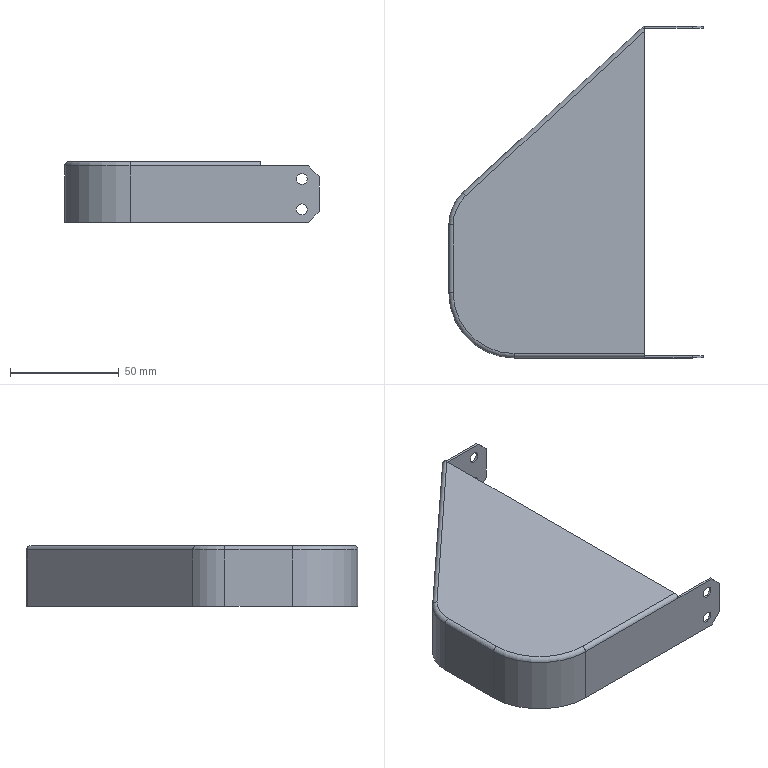Part | STEP file | PN_0003 stopper | 1 solid | 45 faces | box 117 x 152.64 x 28 mm | volume 18137 mm3 | cylinder 20 | plane 20 | torus 4 | sphere 1 | commonest cylinder face diameters 5 x8 2 x4 4 x4 38 x1 40 x1 58 x1